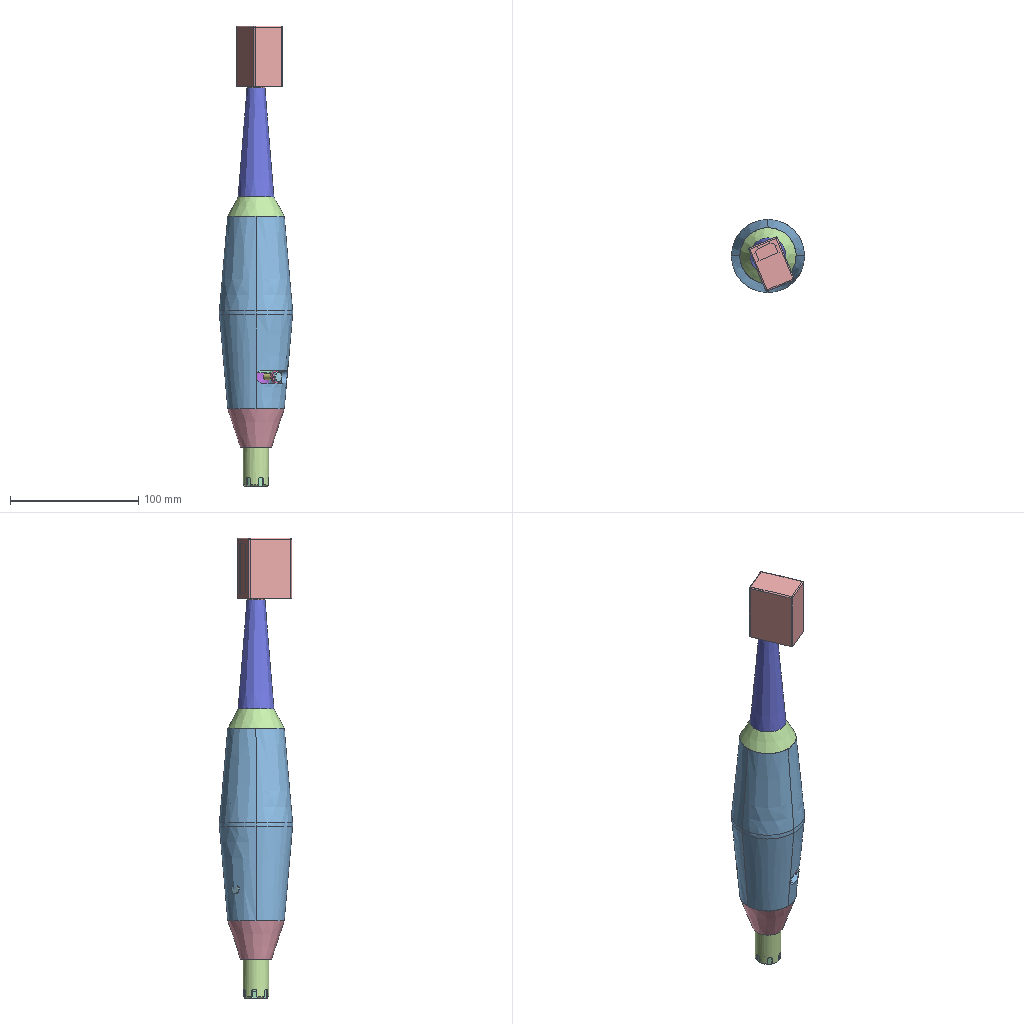Assembly | NX | 31 different items | 64 placed | box 57 x 57 x 358 mm
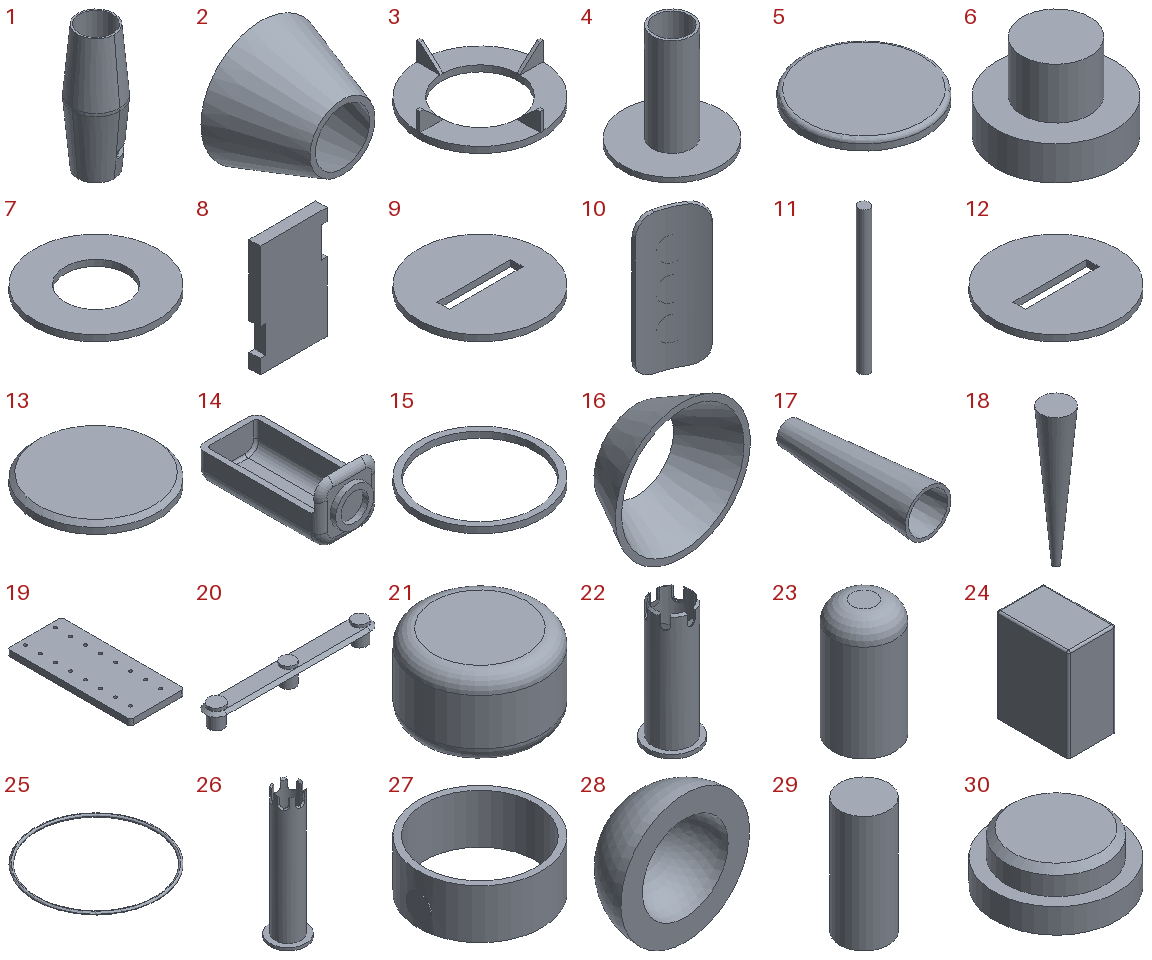Parts list (item | quantity | size | volume | features):
1 | x1 | 57.039 x 57.039 x 150 mm | 113335 mm3 | features EXTRACT_STRING 12, THRU_CURVE_MESH 8, DATUM_CSYS 6, SKETCH 5, LINE 4, Instance Feature 3, Mirror Feature 3, DATUM_PLANE 2, EXTRACT_DATUM_AXIS 2, EXTRACT_DATUM_PLANE 2, EXTRUDE 2, FILL_HOLE 2, BLEND 1, FACE_BLEND 1, SEW 1
2 | x1 | 44 x 30 x 44 mm | 6032 mm3 | features DATUM_CSYS 2, SKETCH 1, SWP104 1
3 | x1 | 40 x 40 x 8 mm | 1634 mm3 | features EXTRUDE 5, EXTRACT_STRING 4, DATUM_CSYS 3, Instance Feature 3, SKETCH 2, Pattern Feature 1
4 | x1 | 40 x 40 x 42 mm | 4398 mm3 | features DATUM_CSYS 3, EXTRUDE 2, SKETCH 2
5 | x1 | 6 x 6 x 0.5 mm | 13.978 mm3 | features DATUM_CSYS 2, BLEND 1, EXTRUDE 1, SKETCH 1
6 | x1 | 35 x 35 x 25 mm | 14334 mm3 | features DATUM_CSYS 3, EXTRUDE 2, SKETCH 2
7 | x1 | 40 x 40 x 2 mm | 1885 mm3 | features DATUM_CSYS 2, EXTRUDE 1, SKETCH 1
8 | x1 | 24 x 4 x 40 mm | 3674 mm3 | features DATUM_CSYS 3, EXTRUDE 2, SKETCH 2
9 | x2 | 40 x 40 x 2 mm | 2321 mm3 | features DATUM_CSYS 2, EXTRUDE 1, SKETCH 1
10 | x1 | 16.263 x 7.446 x 40 mm | 858.511 mm3 | features DATUM_CSYS 3, EXTRUDE 2, SKETCH 2, BLEND 1, DATUM_PLANE 1
11 | x1 | 10 x 10 x 130 mm | 10210 mm3 | features DATUM_CSYS 2, EXTRUDE 1, SKETCH 1
12 | x1 | 40 x 40 x 2 mm | 2321 mm3 | features DATUM_CSYS 2, EXTRUDE 1, SKETCH 1
13 | x1 | 6 x 6 x 0.5 mm | 13.769 mm3 | features DATUM_CSYS 2, CHAMFER 1, EXTRUDE 1, SKETCH 1
14 | x1 | 22 x 47 x 22 mm | 4457 mm3 | features BLEND 5, DATUM_CSYS 4, SKETCH 3, EXTRUDE 2, SHELL 1, SWP104 1
15 | x1 | 40 x 40 x 2 mm | 477.522 mm3 | features DATUM_CSYS 2, EXTRUDE 1, SKETCH 1
16 | x1 | 44 x 15 x 44 mm | 3204 mm3 | features DATUM_CSYS 2, SKETCH 1, SWP104 1
17 | x1 | 28 x 85 x 28 mm | 10147 mm3 | features DATUM_CSYS 2, SWP104 2, SKETCH 1
18 | x24 | 4.85 x 4.85 x 22 mm | 170.37 mm3 | features DATUM_CSYS 3, SKETCH 2, THRU_CURVE 1
19 | x1 | 18 x 41 x 2 mm | 1449 mm3 | features EXTRACT_BODY 7, DATUM_CSYS 3, EXTRUDE 2, SKETCH 2, Pattern Geometry 1, SUBTRACT 1
20 | x8 | 11.5 x 1.5 x 1.4 mm | 5.728 mm3 | features DATUM_CSYS 4, EXTRUDE 3, SKETCH 3, CHAMFER 1
21 | x1 | 40 x 40 x 25 mm | 30143 mm3 | features DATUM_CSYS 2, BLEND 1, EXTRUDE 1, SKETCH 1
22 | x1 | 25 x 25 x 62 mm | 14047 mm3 | features DATUM_CSYS 4, EXTRUDE 3, SKETCH 3, BLEND 2, CHAMFER 2
23 | x1 | 16 x 16 x 30 mm | 1467 mm3 | features DATUM_CSYS 2, BLEND 1, EXTRUDE 1, SHELL 1, SKETCH 1
24 | x1 | 24 x 36.4 x 47 mm | 6181 mm3 | features BLEND 3, DATUM_CSYS 2, EXTRUDE 1, SHELL 1, SKETCH 1
25 | x1 | 40 x 40 x 1 mm | 96.229 mm3 | features DATUM_CSYS 2, BLEND 1, EXTRUDE 1, SKETCH 1
26 | x1 | 25 x 25 x 90 mm | 5042 mm3 | features DATUM_CSYS 5, SKETCH 4, EXTRUDE 3, BLEND 2, CHAMFER 2
27 | x1 | 20 x 20 x 8 mm | 478.886 mm3 | features DATUM_CSYS 3, EXTRUDE 2, SKETCH 2, UNITE 2, Container 1, EXTRACT_BODY 1, Geometry Instance 1
28 | x1 | 6 x 3 x 6 mm | 39.794 mm3 | features DATUM_CSYS 2, SHELL 1, SKETCH 1, SWP104 1
29 | x2 | 5 x 5 x 12 mm | 235.619 mm3 | features DATUM_CSYS 2, EXTRUDE 1, SKETCH 1
30 | x2 | 10 x 10 x 4 mm | 215.33 mm3 | features DATUM_CSYS 3, EXTRUDE 2, SKETCH 2, CHAMFER 1
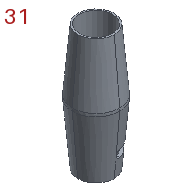31 | x1 | 57.193 x 57.193 x 150 mm | 113335 mm3 | features EXTRACT_STRING 12, THRU_CURVE_MESH 8, DATUM_CSYS 6, SKETCH 5, LINE 4, Instance Feature 3, Mirror Feature 3, DATUM_PLANE 2, EXTRACT_DATUM_AXIS 2, EXTRACT_DATUM_PLANE 2, EXTRUDE 2, FILL_HOLE 2, BLEND 1, FACE_BLEND 1, SEW 1
Mates (type | each side: item.copy, entity, surface, feature):
Bond | 14.1 component | assembly component
Bond | 20.1 component | assembly component | 8 times
Bond | 18.1 component | assembly component | 24 times
LinearPattern | assembly axis | assembly csys | assembly csys | assembly csys | assembly csys | assembly csys | assembly csys | assembly csys | assembly csys | 4 times